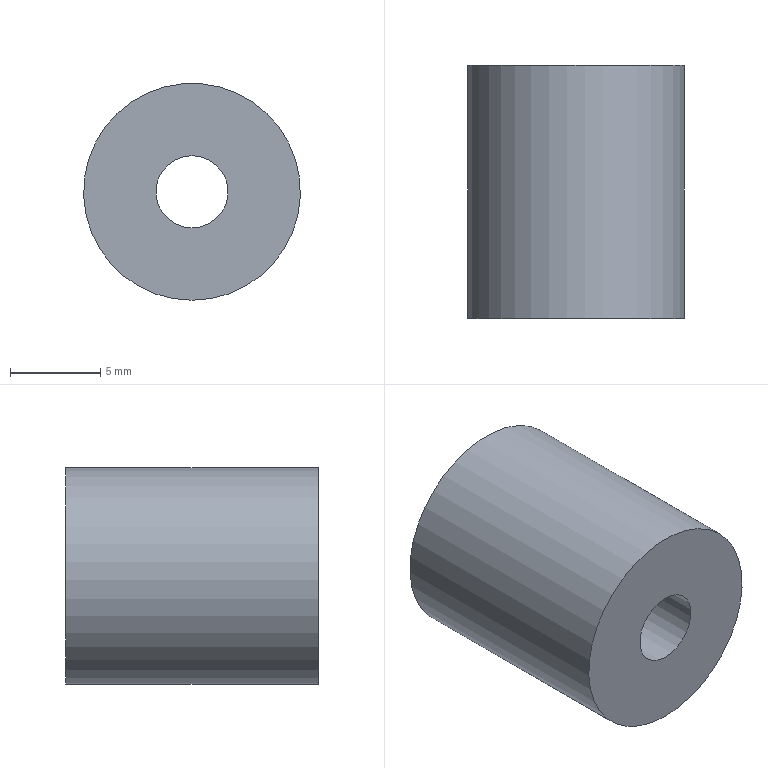Part | STEP file | 1 solid | 6 faces | box 12 x 14 x 12 mm | volume 1266 mm3 | cylinder 3 | plane 3 | commonest cylinder face diameters 4 x1 6 x1 12 x1
STEP:
#1=CARTESIAN_POINT('',(0.,0.,0.));
#2=DIRECTION('',(0.,0.,1.));
#3=DIRECTION('',(1.,0.,0.));
#4=AXIS2_PLACEMENT_3D('',#1,#2,#3);
#5=CARTESIAN_POINT('',(0.,0.,-6.));
#6=VERTEX_POINT('',#5);
#7=CARTESIAN_POINT('',(0.,0.,0.));
#8=DIRECTION('',(0.,1.,0.));
#9=DIRECTION('',(0.,0.,-1.));
#10=AXIS2_PLACEMENT_3D('',#7,#8,#9);
#11=CIRCLE('',#10,6.);
#12=CARTESIAN_POINT('',(0.,0.,0.));
#13=DIRECTION('',(0.,-1.,0.));
#14=DIRECTION('',(0.,0.,-1.));
#15=AXIS2_PLACEMENT_3D('',#12,#13,#14);
#16=CYLINDRICAL_SURFACE('',#15,6.);
#17=CARTESIAN_POINT('',(6.283,0.));
#18=DIRECTION('',(-1.,0.));
#19=VECTOR('',#18,1.);
#20=LINE('',#17,#19);
#21=(GEOMETRIC_REPRESENTATION_CONTEXT(2)PARAMETRIC_REPRESENTATION_CONTEXT()REPRESENTATION_CONTEXT('',''));
#22=DEFINITIONAL_REPRESENTATION('',(#20),#21);
#23=PCURVE('',#16,#22);
#24=CARTESIAN_POINT('',(0.,0.,2.));
#25=DIRECTION('',(0.,1.,0.));
#26=DIRECTION('',(0.,0.,1.));
#27=AXIS2_PLACEMENT_3D('',#24,#25,#26);
#28=PLANE('',#27);
#29=CARTESIAN_POINT('',(-2.,0.));
#30=DIRECTION('',(-1.,0.));
#31=AXIS2_PLACEMENT_2D('',#29,#30);
#32=CIRCLE('',#31,6.);
#33=(GEOMETRIC_REPRESENTATION_CONTEXT(2)PARAMETRIC_REPRESENTATION_CONTEXT()REPRESENTATION_CONTEXT('',''));
#34=DEFINITIONAL_REPRESENTATION('',(#32),#33);
#35=PCURVE('',#28,#34);
#36=SURFACE_CURVE('',#11,(#23,#35),.PCURVE_S1.);
#37=EDGE_CURVE('',#6,#6,#36,.T.);
#38=ORIENTED_EDGE('',*,*,#37,.T.);
#39=CARTESIAN_POINT('',(0.,14.,-6.));
#40=VERTEX_POINT('',#39);
#41=CARTESIAN_POINT('',(0.,14.,-6.));
#42=CARTESIAN_POINT('',(0.,0.,-6.));
#43=B_SPLINE_CURVE_WITH_KNOTS('',1,(#41,#42),.UNSPECIFIED.,.F.,.F.,(2,2),(-14.,0.),.PIECEWISE_BEZIER_KNOTS.);
#44=CARTESIAN_POINT('',(0.,0.));
#45=DIRECTION('',(0.,1.));
#46=VECTOR('',#45,1.);
#47=LINE('',#44,#46);
#48=(GEOMETRIC_REPRESENTATION_CONTEXT(2)PARAMETRIC_REPRESENTATION_CONTEXT()REPRESENTATION_CONTEXT('',''));
#49=DEFINITIONAL_REPRESENTATION('',(#47),#48);
#50=PCURVE('',#16,#49);
#51=CARTESIAN_POINT('',(6.283,0.));
#52=DIRECTION('',(0.,1.));
#53=VECTOR('',#52,1.);
#54=LINE('',#51,#53);
#55=(GEOMETRIC_REPRESENTATION_CONTEXT(2)PARAMETRIC_REPRESENTATION_CONTEXT()REPRESENTATION_CONTEXT('',''));
#56=DEFINITIONAL_REPRESENTATION('',(#54),#55);
#57=PCURVE('',#16,#56);
#58=SEAM_CURVE('',#43,(#50,#57),.PCURVE_S1.);
#59=EDGE_CURVE('',#40,#6,#58,.T.);
#60=ORIENTED_EDGE('',*,*,#59,.F.);
#61=CARTESIAN_POINT('',(0.,14.,0.));
#62=DIRECTION('',(0.,-1.,0.));
#63=DIRECTION('',(0.,0.,-1.));
#64=AXIS2_PLACEMENT_3D('',#61,#62,#63);
#65=CIRCLE('',#64,6.);
#66=CARTESIAN_POINT('',(0.,-14.));
#67=DIRECTION('',(1.,0.));
#68=VECTOR('',#67,1.);
#69=LINE('',#66,#68);
#70=(GEOMETRIC_REPRESENTATION_CONTEXT(2)PARAMETRIC_REPRESENTATION_CONTEXT()REPRESENTATION_CONTEXT('',''));
#71=DEFINITIONAL_REPRESENTATION('',(#69),#70);
#72=PCURVE('',#16,#71);
#73=CARTESIAN_POINT('',(0.,14.,3.));
#74=DIRECTION('',(0.,-1.,0.));
#75=DIRECTION('',(0.,0.,-1.));
#76=AXIS2_PLACEMENT_3D('',#73,#74,#75);
#77=PLANE('',#76);
#78=CARTESIAN_POINT('',(3.,0.));
#79=DIRECTION('',(1.,0.));
#80=AXIS2_PLACEMENT_2D('',#78,#79);
#81=CIRCLE('',#80,6.);
#82=(GEOMETRIC_REPRESENTATION_CONTEXT(2)PARAMETRIC_REPRESENTATION_CONTEXT()REPRESENTATION_CONTEXT('',''));
#83=DEFINITIONAL_REPRESENTATION('',(#81),#82);
#84=PCURVE('',#77,#83);
#85=SURFACE_CURVE('',#65,(#72,#84),.PCURVE_S1.);
#86=EDGE_CURVE('',#40,#40,#85,.T.);
#87=ORIENTED_EDGE('',*,*,#86,.T.);
#88=ORIENTED_EDGE('',*,*,#59,.T.);
#89=EDGE_LOOP('',(#38,#60,#87,#88));
#90=FACE_BOUND('',#89,.T.);
#91=ADVANCED_FACE('',(#90),#16,.T.);
#92=CARTESIAN_POINT('',(0.,0.,-2.));
#93=VERTEX_POINT('',#92);
#94=CARTESIAN_POINT('',(0.,0.,0.));
#95=DIRECTION('',(0.,-1.,0.));
#96=DIRECTION('',(0.,0.,-1.));
#97=AXIS2_PLACEMENT_3D('',#94,#95,#96);
#98=CIRCLE('',#97,2.);
#99=CARTESIAN_POINT('',(-4.,0.));
#100=CARTESIAN_POINT('',(-4.,3.464));
#101=CARTESIAN_POINT('',(-1.,1.732));
#102=CARTESIAN_POINT('',(2.,0.));
#103=CARTESIAN_POINT('',(-1.,-1.732));
#104=CARTESIAN_POINT('',(-4.,-3.464));
#105=CARTESIAN_POINT('',(-4.,0.));
#106=(BOUNDED_CURVE()B_SPLINE_CURVE(2,(#99,#100,#101,#102,#103,#104,#105),.UNSPECIFIED.,.T.,.F.)B_SPLINE_CURVE_WITH_KNOTS((1,2,2,2,2,1),(-2.094,0.,2.094,4.189,6.283,8.378),.UNSPECIFIED.)CURVE()GEOMETRIC_REPRESENTATION_ITEM()RATIONAL_B_SPLINE_CURVE((1.,0.5,1.,0.5,1.,0.5,1.))REPRESENTATION_ITEM(''));
#107=(GEOMETRIC_REPRESENTATION_CONTEXT(2)PARAMETRIC_REPRESENTATION_CONTEXT()REPRESENTATION_CONTEXT('',''));
#108=DEFINITIONAL_REPRESENTATION('',(#106),#107);
#109=PCURVE('',#28,#108);
#110=CARTESIAN_POINT('',(0.,0.,0.));
#111=DIRECTION('',(0.,-1.,0.));
#112=DIRECTION('',(0.,0.,-1.));
#113=AXIS2_PLACEMENT_3D('',#110,#111,#112);
#114=CYLINDRICAL_SURFACE('',#113,2.);
#115=CARTESIAN_POINT('',(0.,0.));
#116=DIRECTION('',(1.,0.));
#117=VECTOR('',#116,1.);
#118=LINE('',#115,#117);
#119=(GEOMETRIC_REPRESENTATION_CONTEXT(2)PARAMETRIC_REPRESENTATION_CONTEXT()REPRESENTATION_CONTEXT('',''));
#120=DEFINITIONAL_REPRESENTATION('',(#118),#119);
#121=PCURVE('',#114,#120);
#122=SURFACE_CURVE('',#98,(#109,#121),.PCURVE_S1.);
#123=EDGE_CURVE('',#93,#93,#122,.T.);
#124=ORIENTED_EDGE('',*,*,#123,.F.);
#125=EDGE_LOOP('',(#124));
#126=FACE_BOUND('',#125,.T.);
#127=ORIENTED_EDGE('',*,*,#37,.F.);
#128=EDGE_LOOP('',(#127));
#129=FACE_BOUND('',#128,.T.);
#130=ADVANCED_FACE('',(#126,#129),#28,.F.);
#131=CARTESIAN_POINT('',(0.,14.,-3.));
#132=VERTEX_POINT('',#131);
#133=CARTESIAN_POINT('',(0.,14.,0.));
#134=DIRECTION('',(0.,1.,0.));
#135=DIRECTION('',(0.,0.,-1.));
#136=AXIS2_PLACEMENT_3D('',#133,#134,#135);
#137=CIRCLE('',#136,3.);
#138=CARTESIAN_POINT('',(6.,0.));
#139=CARTESIAN_POINT('',(6.,-5.196));
#140=CARTESIAN_POINT('',(1.5,-2.598));
#141=CARTESIAN_POINT('',(-3.,0.));
#142=CARTESIAN_POINT('',(1.5,2.598));
#143=CARTESIAN_POINT('',(6.,5.196));
#144=CARTESIAN_POINT('',(6.,0.));
#145=(BOUNDED_CURVE()B_SPLINE_CURVE(2,(#138,#139,#140,#141,#142,#143,#144),.UNSPECIFIED.,.T.,.F.)B_SPLINE_CURVE_WITH_KNOTS((1,2,2,2,2,1),(-2.094,0.,2.094,4.189,6.283,8.378),.UNSPECIFIED.)CURVE()GEOMETRIC_REPRESENTATION_ITEM()RATIONAL_B_SPLINE_CURVE((1.,0.5,1.,0.5,1.,0.5,1.))REPRESENTATION_ITEM(''));
#146=(GEOMETRIC_REPRESENTATION_CONTEXT(2)PARAMETRIC_REPRESENTATION_CONTEXT()REPRESENTATION_CONTEXT('',''));
#147=DEFINITIONAL_REPRESENTATION('',(#145),#146);
#148=PCURVE('',#77,#147);
#149=CARTESIAN_POINT('',(0.,0.,0.));
#150=DIRECTION('',(0.,-1.,0.));
#151=DIRECTION('',(0.,0.,-1.));
#152=AXIS2_PLACEMENT_3D('',#149,#150,#151);
#153=CYLINDRICAL_SURFACE('',#152,3.);
#154=CARTESIAN_POINT('',(6.283,-14.));
#155=DIRECTION('',(-1.,0.));
#156=VECTOR('',#155,1.);
#157=LINE('',#154,#156);
#158=(GEOMETRIC_REPRESENTATION_CONTEXT(2)PARAMETRIC_REPRESENTATION_CONTEXT()REPRESENTATION_CONTEXT('',''));
#159=DEFINITIONAL_REPRESENTATION('',(#157),#158);
#160=PCURVE('',#153,#159);
#161=SURFACE_CURVE('',#137,(#148,#160),.PCURVE_S1.);
#162=EDGE_CURVE('',#132,#132,#161,.T.);
#163=ORIENTED_EDGE('',*,*,#162,.F.);
#164=EDGE_LOOP('',(#163));
#165=FACE_BOUND('',#164,.T.);
#166=ORIENTED_EDGE('',*,*,#86,.F.);
#167=EDGE_LOOP('',(#166));
#168=FACE_BOUND('',#167,.T.);
#169=ADVANCED_FACE('',(#165,#168),#77,.F.);
#170=CARTESIAN_POINT('',(0.,5.,-2.));
#171=VERTEX_POINT('',#170);
#172=CARTESIAN_POINT('',(0.,5.,0.));
#173=DIRECTION('',(0.,-1.,0.));
#174=DIRECTION('',(0.,0.,-1.));
#175=AXIS2_PLACEMENT_3D('',#172,#173,#174);
#176=CIRCLE('',#175,2.);
#177=CARTESIAN_POINT('',(0.,-5.));
#178=DIRECTION('',(1.,0.));
#179=VECTOR('',#178,1.);
#180=LINE('',#177,#179);
#181=(GEOMETRIC_REPRESENTATION_CONTEXT(2)PARAMETRIC_REPRESENTATION_CONTEXT()REPRESENTATION_CONTEXT('',''));
#182=DEFINITIONAL_REPRESENTATION('',(#180),#181);
#183=PCURVE('',#114,#182);
#184=CARTESIAN_POINT('',(0.,5.,2.));
#185=DIRECTION('',(0.,-1.,0.));
#186=DIRECTION('',(0.,0.,-1.));
#187=AXIS2_PLACEMENT_3D('',#184,#185,#186);
#188=PLANE('',#187);
#189=CARTESIAN_POINT('',(2.,0.));
#190=DIRECTION('',(1.,0.));
#191=AXIS2_PLACEMENT_2D('',#189,#190);
#192=CIRCLE('',#191,2.);
#193=(GEOMETRIC_REPRESENTATION_CONTEXT(2)PARAMETRIC_REPRESENTATION_CONTEXT()REPRESENTATION_CONTEXT('',''));
#194=DEFINITIONAL_REPRESENTATION('',(#192),#193);
#195=PCURVE('',#188,#194);
#196=SURFACE_CURVE('',#176,(#183,#195),.PCURVE_S1.);
#197=EDGE_CURVE('',#171,#171,#196,.T.);
#198=ORIENTED_EDGE('',*,*,#197,.T.);
#199=CARTESIAN_POINT('',(0.,5.,-2.));
#200=CARTESIAN_POINT('',(0.,0.,-2.));
#201=B_SPLINE_CURVE_WITH_KNOTS('',1,(#199,#200),.UNSPECIFIED.,.F.,.F.,(2,2),(-5.,0.),.PIECEWISE_BEZIER_KNOTS.);
#202=CARTESIAN_POINT('',(6.283,0.));
#203=DIRECTION('',(0.,1.));
#204=VECTOR('',#203,1.);
#205=LINE('',#202,#204);
#206=(GEOMETRIC_REPRESENTATION_CONTEXT(2)PARAMETRIC_REPRESENTATION_CONTEXT()REPRESENTATION_CONTEXT('',''));
#207=DEFINITIONAL_REPRESENTATION('',(#205),#206);
#208=PCURVE('',#114,#207);
#209=CARTESIAN_POINT('',(0.,0.));
#210=DIRECTION('',(0.,1.));
#211=VECTOR('',#210,1.);
#212=LINE('',#209,#211);
#213=(GEOMETRIC_REPRESENTATION_CONTEXT(2)PARAMETRIC_REPRESENTATION_CONTEXT()REPRESENTATION_CONTEXT('',''));
#214=DEFINITIONAL_REPRESENTATION('',(#212),#213);
#215=PCURVE('',#114,#214);
#216=SEAM_CURVE('',#201,(#208,#215),.PCURVE_S1.);
#217=EDGE_CURVE('',#171,#93,#216,.T.);
#218=ORIENTED_EDGE('',*,*,#217,.T.);
#219=ORIENTED_EDGE('',*,*,#123,.F.);
#220=ORIENTED_EDGE('',*,*,#217,.F.);
#221=EDGE_LOOP('',(#198,#218,#219,#220));
#222=FACE_BOUND('',#221,.F.);
#223=ADVANCED_FACE('',(#222),#114,.F.);
#224=ORIENTED_EDGE('',*,*,#162,.F.);
#225=CARTESIAN_POINT('',(0.,5.,-3.));
#226=VERTEX_POINT('',#225);
#227=CARTESIAN_POINT('',(0.,14.,-3.));
#228=CARTESIAN_POINT('',(0.,5.,-3.));
#229=B_SPLINE_CURVE_WITH_KNOTS('',1,(#227,#228),.UNSPECIFIED.,.F.,.F.,(2,2),(-14.,-5.),.PIECEWISE_BEZIER_KNOTS.);
#230=CARTESIAN_POINT('',(6.283,0.));
#231=DIRECTION('',(0.,1.));
#232=VECTOR('',#231,1.);
#233=LINE('',#230,#232);
#234=(GEOMETRIC_REPRESENTATION_CONTEXT(2)PARAMETRIC_REPRESENTATION_CONTEXT()REPRESENTATION_CONTEXT('',''));
#235=DEFINITIONAL_REPRESENTATION('',(#233),#234);
#236=PCURVE('',#153,#235);
#237=CARTESIAN_POINT('',(0.,0.));
#238=DIRECTION('',(0.,1.));
#239=VECTOR('',#238,1.);
#240=LINE('',#237,#239);
#241=(GEOMETRIC_REPRESENTATION_CONTEXT(2)PARAMETRIC_REPRESENTATION_CONTEXT()REPRESENTATION_CONTEXT('',''));
#242=DEFINITIONAL_REPRESENTATION('',(#240),#241);
#243=PCURVE('',#153,#242);
#244=SEAM_CURVE('',#229,(#236,#243),.PCURVE_S1.);
#245=EDGE_CURVE('',#132,#226,#244,.T.);
#246=ORIENTED_EDGE('',*,*,#245,.T.);
#247=CARTESIAN_POINT('',(0.,5.,0.));
#248=DIRECTION('',(0.,1.,0.));
#249=DIRECTION('',(0.,0.,-1.));
#250=AXIS2_PLACEMENT_3D('',#247,#248,#249);
#251=CIRCLE('',#250,3.);
#252=CARTESIAN_POINT('',(6.283,-5.));
#253=DIRECTION('',(-1.,0.));
#254=VECTOR('',#253,1.);
#255=LINE('',#252,#254);
#256=(GEOMETRIC_REPRESENTATION_CONTEXT(2)PARAMETRIC_REPRESENTATION_CONTEXT()REPRESENTATION_CONTEXT('',''));
#257=DEFINITIONAL_REPRESENTATION('',(#255),#256);
#258=PCURVE('',#153,#257);
#259=CARTESIAN_POINT('',(5.,0.));
#260=CARTESIAN_POINT('',(5.,-5.196));
#261=CARTESIAN_POINT('',(0.5,-2.598));
#262=CARTESIAN_POINT('',(-4.,0.));
#263=CARTESIAN_POINT('',(0.5,2.598));
#264=CARTESIAN_POINT('',(5.,5.196));
#265=CARTESIAN_POINT('',(5.,0.));
#266=(BOUNDED_CURVE()B_SPLINE_CURVE(2,(#259,#260,#261,#262,#263,#264,#265),.UNSPECIFIED.,.T.,.F.)B_SPLINE_CURVE_WITH_KNOTS((1,2,2,2,2,1),(-2.094,0.,2.094,4.189,6.283,8.378),.UNSPECIFIED.)CURVE()GEOMETRIC_REPRESENTATION_ITEM()RATIONAL_B_SPLINE_CURVE((1.,0.5,1.,0.5,1.,0.5,1.))REPRESENTATION_ITEM(''));
#267=(GEOMETRIC_REPRESENTATION_CONTEXT(2)PARAMETRIC_REPRESENTATION_CONTEXT()REPRESENTATION_CONTEXT('',''));
#268=DEFINITIONAL_REPRESENTATION('',(#266),#267);
#269=PCURVE('',#188,#268);
#270=SURFACE_CURVE('',#251,(#258,#269),.PCURVE_S1.);
#271=EDGE_CURVE('',#226,#226,#270,.T.);
#272=ORIENTED_EDGE('',*,*,#271,.T.);
#273=ORIENTED_EDGE('',*,*,#245,.F.);
#274=EDGE_LOOP('',(#224,#246,#272,#273));
#275=FACE_BOUND('',#274,.F.);
#276=ADVANCED_FACE('',(#275),#153,.F.);
#277=ORIENTED_EDGE('',*,*,#197,.T.);
#278=EDGE_LOOP('',(#277));
#279=FACE_BOUND('',#278,.T.);
#280=ORIENTED_EDGE('',*,*,#271,.T.);
#281=EDGE_LOOP('',(#280));
#282=FACE_BOUND('',#281,.T.);
#283=ADVANCED_FACE('',(#279,#282),#188,.F.);
#284=CLOSED_SHELL('',(#91,#130,#169,#223,#276,#283));
#285=MANIFOLD_SOLID_BREP('',#284);
#286=(LENGTH_UNIT()NAMED_UNIT(*)SI_UNIT(.MILLI.,.METRE.));
#287=UNCERTAINTY_MEASURE_WITH_UNIT(LENGTH_MEASURE(0.00001),#286,'','');
#288=(NAMED_UNIT(*)PLANE_ANGLE_UNIT()SI_UNIT($,.RADIAN.));
#289=(NAMED_UNIT(*)SI_UNIT($,.STERADIAN.)SOLID_ANGLE_UNIT());
#290=(GEOMETRIC_REPRESENTATION_CONTEXT(3)GLOBAL_UNCERTAINTY_ASSIGNED_CONTEXT((#287))GLOBAL_UNIT_ASSIGNED_CONTEXT((#286,#288,#289))REPRESENTATION_CONTEXT('',''));
#291=ADVANCED_BREP_SHAPE_REPRESENTATION('',(#4,#285),#290);